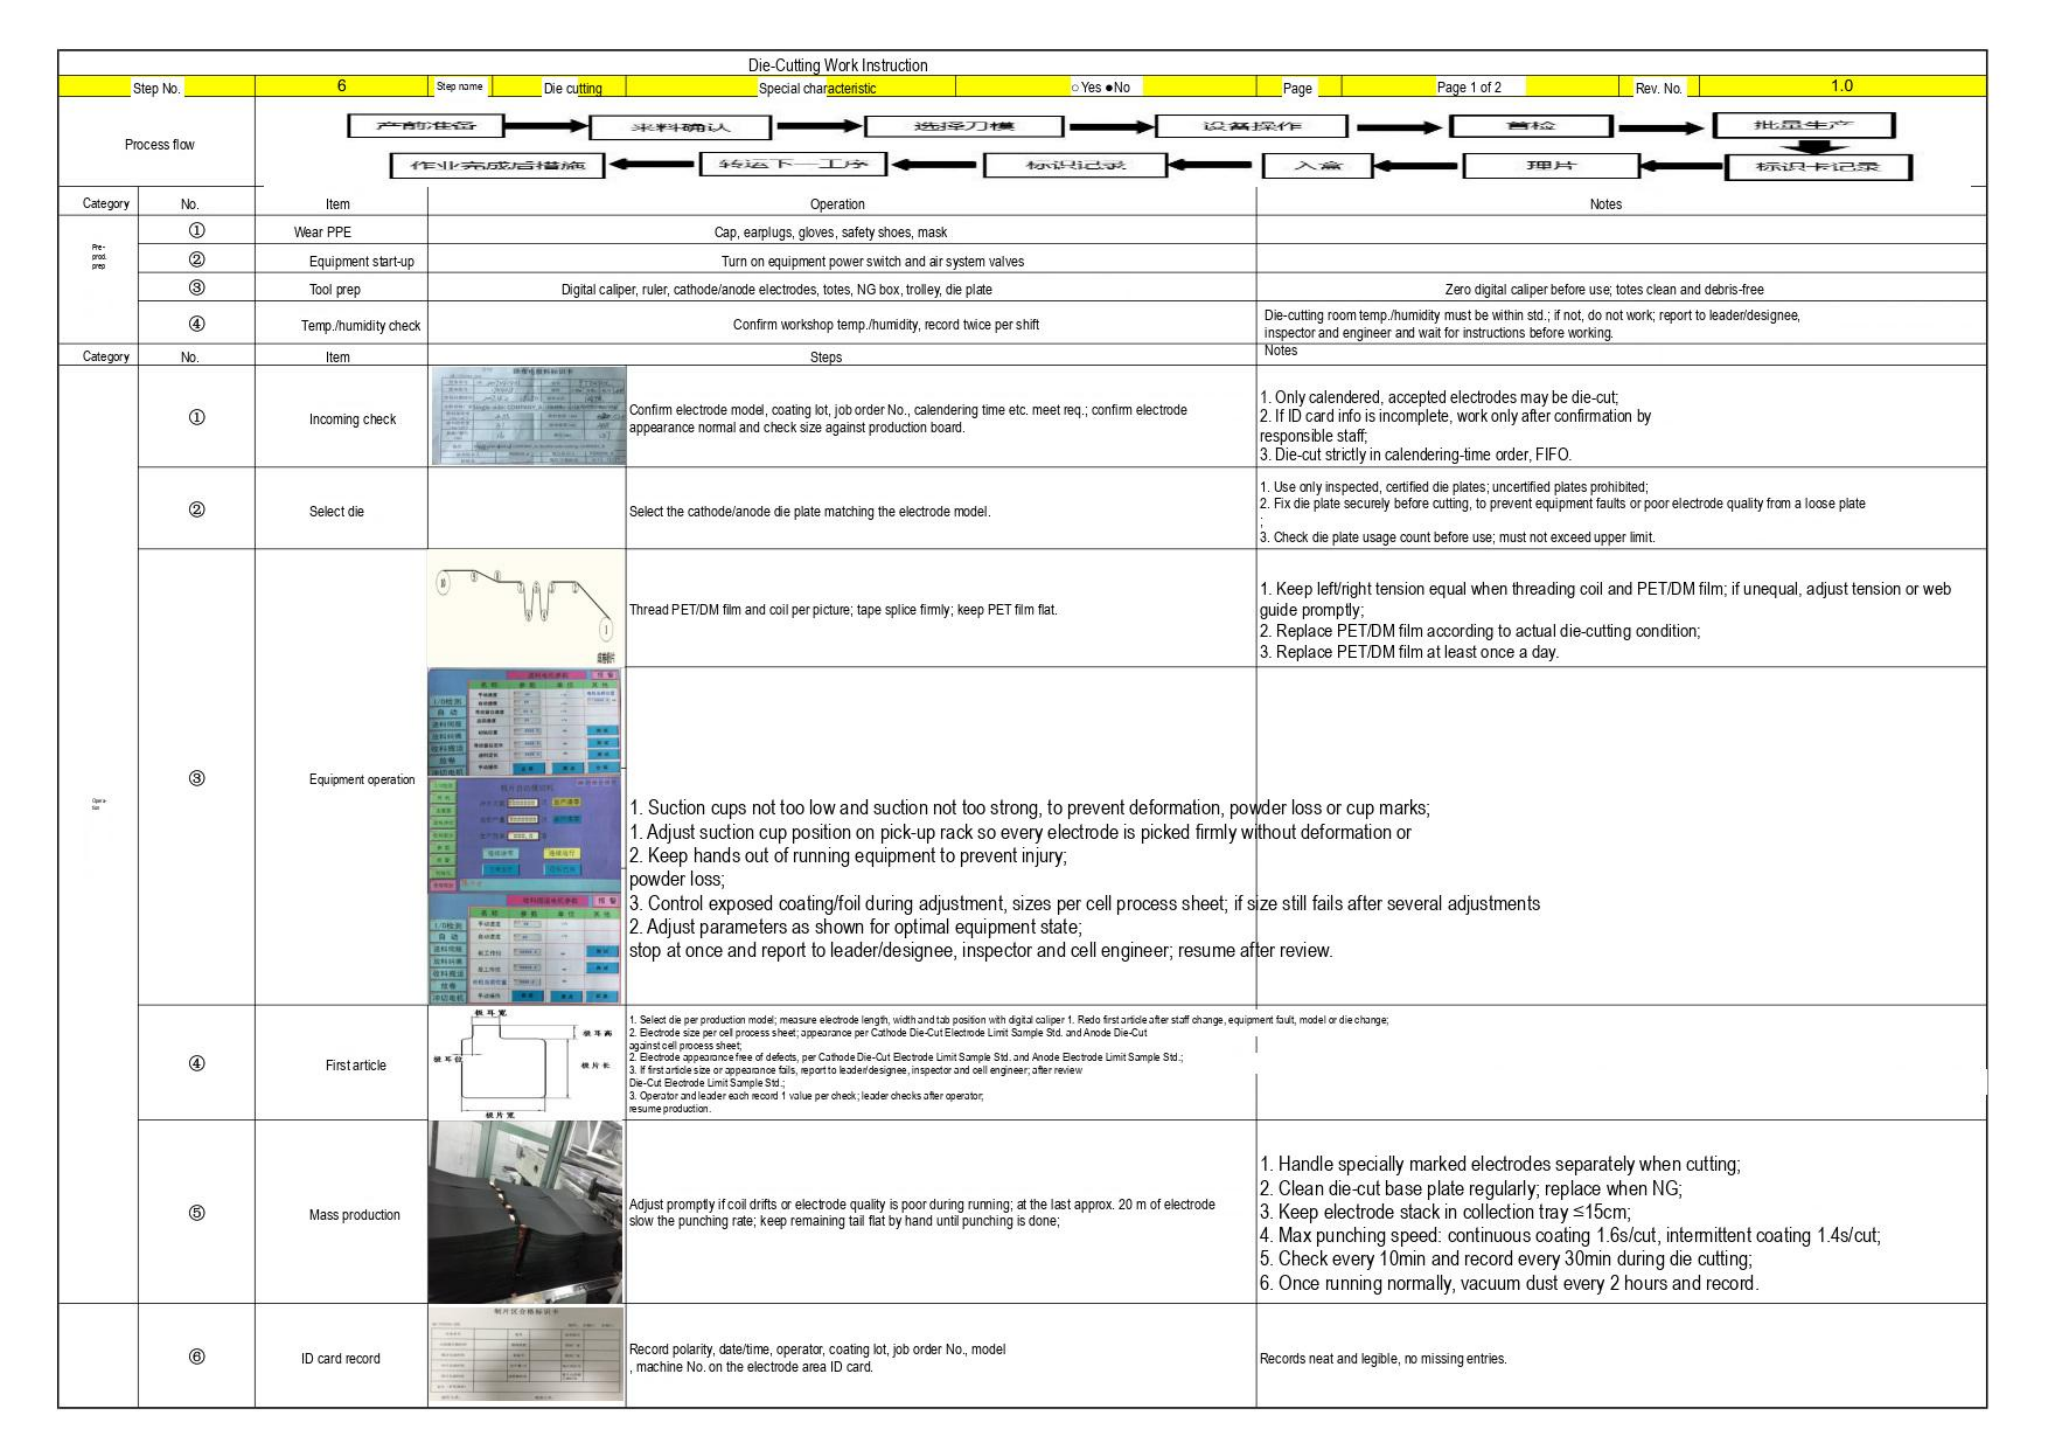Die-Cutting Work Instruction

| Step No. | 6 | Step name | Die cutting | Special characteristic | ○Yes ●No | Page | Page 1 of 2 | Rev. No. | 1.0 |
|---|---|---|---|---|---|---|---|---|---|

Process flow

产前准备 → 来料确认 → 选择刀模 → 设备操作 → 首检 → 批量生产 → 标识卡记录 → 理片 → 入篮 → 标识记录 → 转运下一工序 → 作业完成后措施

| Category | No. | Item | Operation | Notes |
|---|---|---|---|---|
| Pre-prod. prep | ① | Wear PPE | Cap, earplugs, gloves, safety shoes, mask | |
| | ② | Equipment start-up | Turn on equipment power switch and air system valves | |
| | ③ | Tool prep | Digital caliper, ruler, cathode/anode electrodes, totes, NG box, trolley, die plate | Zero digital caliper before use; totes clean and debris-free |
| | ④ | Temp./humidity check | Confirm workshop temp./humidity, record twice per shift | Die-cutting room temp./humidity must be within std.; if not, do not work; report to leader/designee, inspector and engineer and wait for instructions before working. |

| Category | No. | Item | Steps | Notes |
|---|---|---|---|---|
| | ① | Incoming check | Confirm electrode model, coating lot, job order No., calendering time etc. meet req.; confirm electrode appearance normal and check size against production board. | 1. Only calendered, accepted electrodes may be die-cut;<br>2. If ID card info is incomplete, work only after confirmation by responsible staff;<br>3. Die-cut strictly in calendering-time order, FIFO. |
| | ② | Select die | Select the cathode/anode die plate matching the electrode model. | 1. Use only inspected, certified die plates; uncertified plates prohibited;<br>2. Fix die plate securely before cutting, to prevent equipment faults or poor electrode quality from a loose plate<br>;<br>3. Check die plate usage count before use; must not exceed upper limit. |
| | ③ | Equipment operation | Thread PET/DM film and coil per picture; tape splice firmly; keep PET film flat. | 1. Keep left/right tension equal when threading coil and PET/DM film; if unequal, adjust tension or web guide promptly;<br>2. Replace PET/DM film according to actual die-cutting condition;<br>3. Replace PET/DM film at least once a day. |
| | | | 1. Suction cups not too low and suction not too strong, to prevent deformation, powder loss or cup marks;<br>1. Adjust suction cup position on pick-up rack so every electrode is picked firmly without deformation or<br>2. Keep hands out of running equipment to prevent injury;<br>powder loss;<br>3. Control exposed coating/foil during adjustment, sizes per cell process sheet; if size still fails after several adjustments<br>2. Adjust parameters as shown for optimal equipment state;<br>stop at once and report to leader/designee, inspector and cell engineer; resume after review. | |
| | ④ | First article | 极耳宽<br>极耳高<br>极耳位<br>极片长<br>极片宽<br>1. Select die per production model; measure electrode length, width and tab position with digital caliper 1. Redo first article after staff change, equipment fault, model or die change;<br>2. Electrode size per cell process sheet; appearance per Cathode Die-Cut Electrode Limit Sample Std. and Anode Die-Cut<br>against cell process sheet;<br>2. Electrode appearance free of defects, per Cathode Die-Cut Electrode Limit Sample Std. and Anode Electrode Limit Sample Std.;<br>3. If first article size or appearance fails, report to leader/designee, inspector and cell engineer; after review<br>Die-Cut Electrode Limit Sample Std.;<br>3. Operator and leader each record 1 value per check; leader checks after operator;<br>resume production. | |
| | ⑤ | Mass production | Adjust promptly if coil drifts or electrode quality is poor during running; at the last approx. 20 m of electrode slow the punching rate; keep remaining tail flat by hand until punching is done; | 1. Handle specially marked electrodes separately when cutting;<br>2. Clean die-cut base plate regularly; replace when NG;<br>3. Keep electrode stack in collection tray ≤15cm;<br>4. Max punching speed: continuous coating 1.6s/cut, intermittent coating 1.4s/cut;<br>5. Check every 10min and record every 30min during die cutting;<br>6. Once running normally, vacuum dust every 2 hours and record. |
| | ⑥ | ID card record | Record polarity, date/time, operator, coating lot, job order No., model<br>, machine No. on the electrode area ID card. | Records neat and legible, no missing entries. |
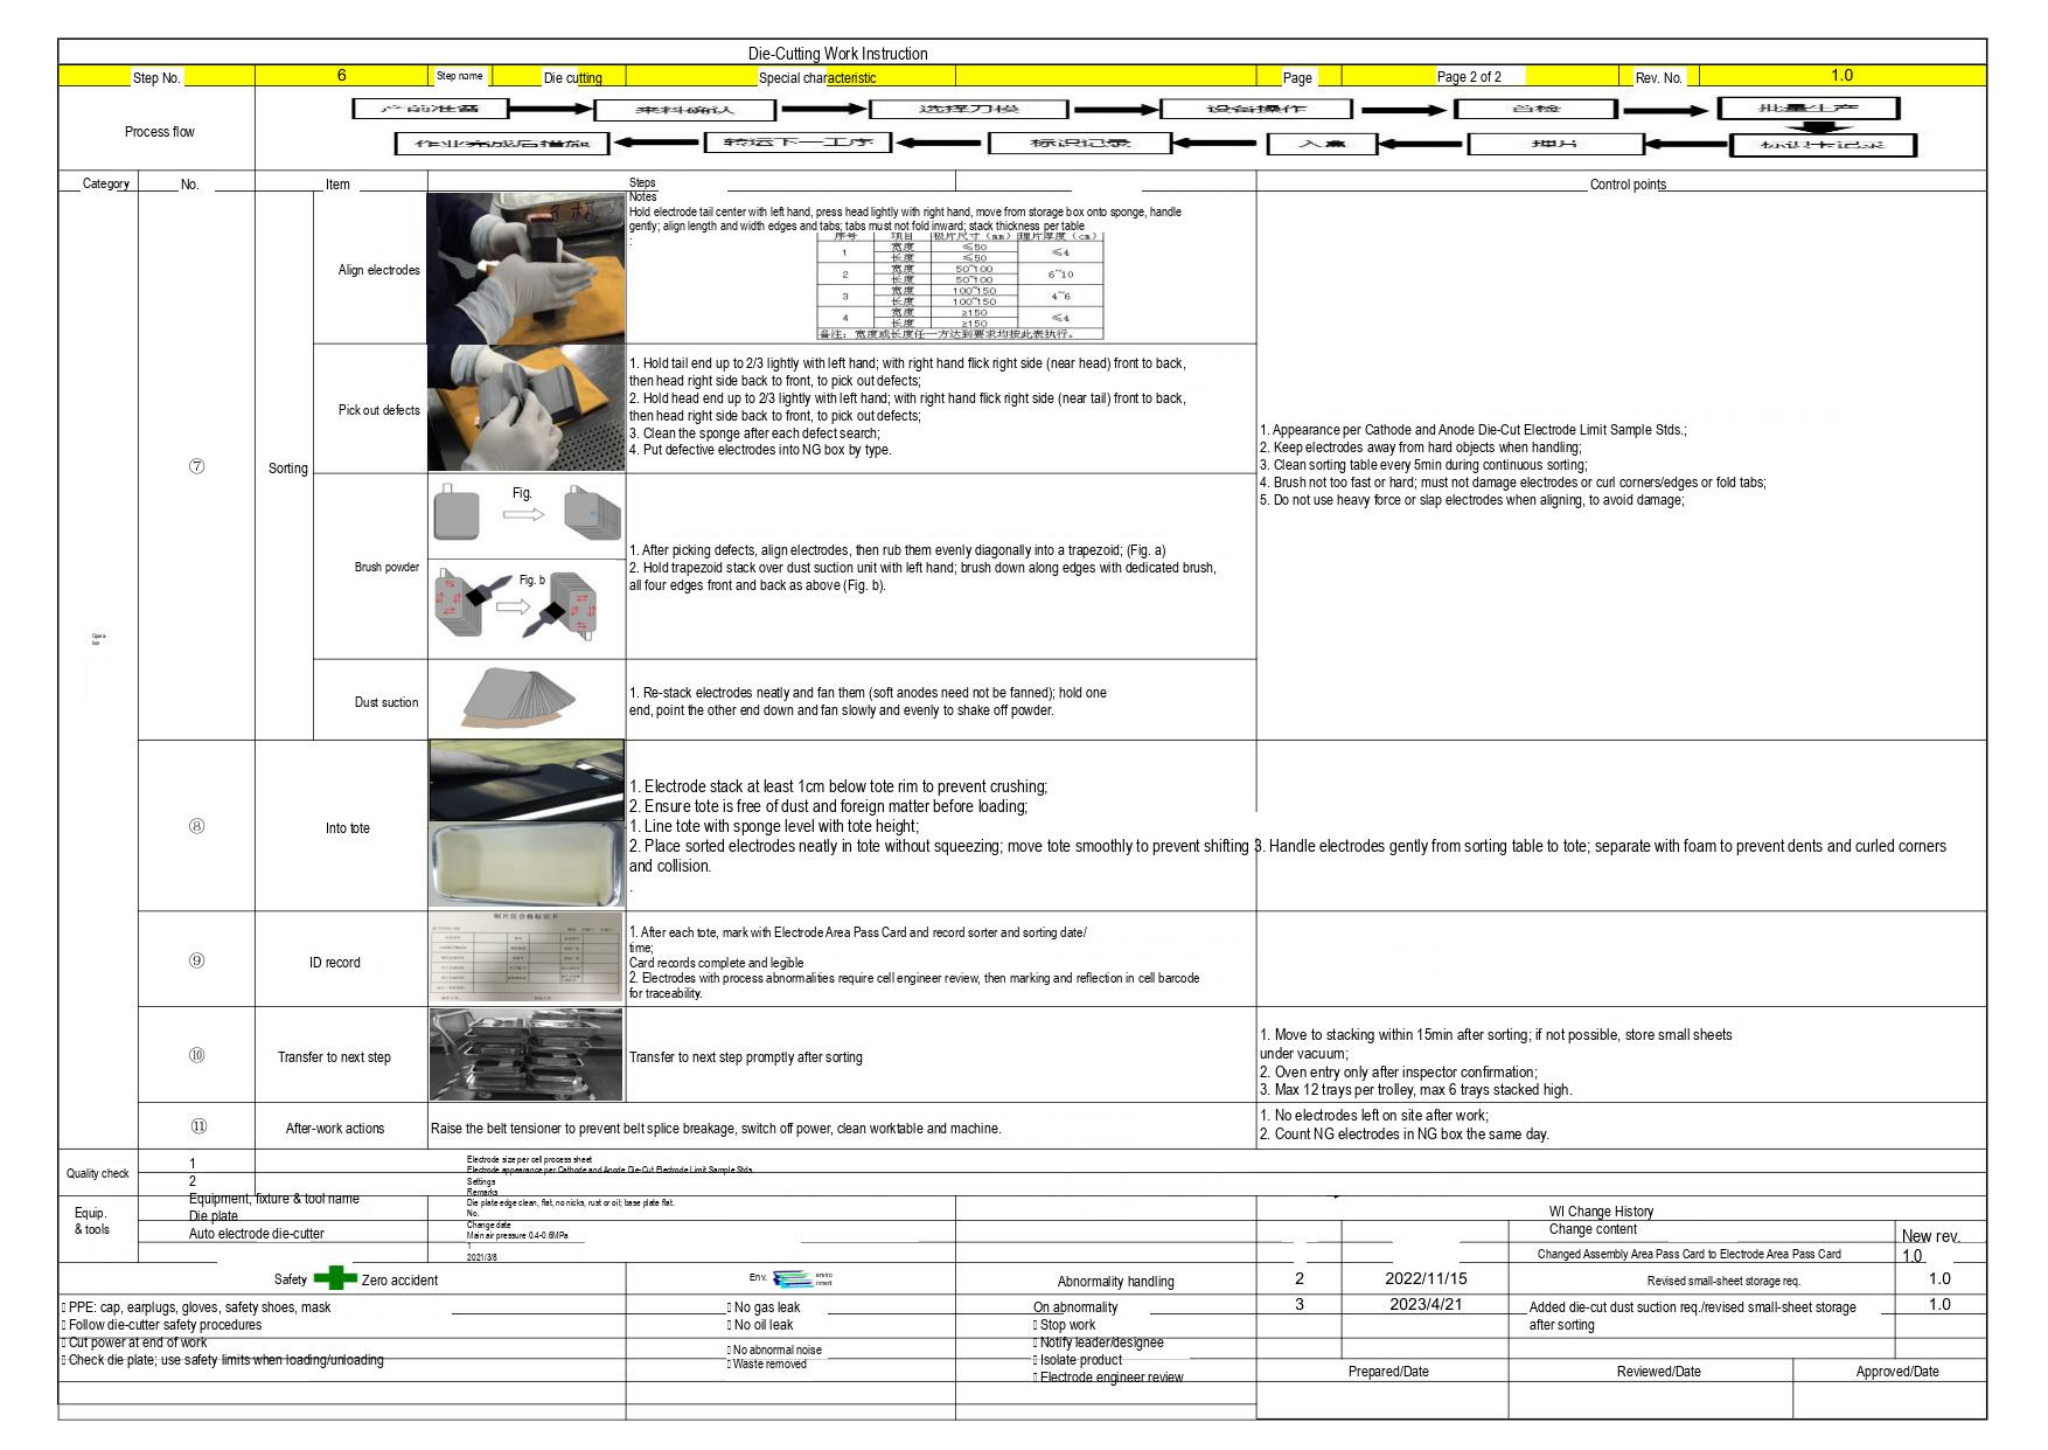# Die-Cutting Work Instruction

| Step No. | 6 | Step name | Die cutting | Special characteristic | | Page | Page 2 of 2 | Rev. No. | 1.0 |
|---|---|---|---|---|---|---|---|---|---|

**Process flow**

来料确认 → 选择刀模 → 设备操作 → 自检 → 批量生产

作业完成后措施 ← 转运下一工序 ← 标识记录 ← 入库 ← 抽片

| Category | No. | Item | | Steps / Notes | Control points |
|---|---|---|---|---|---|
| | ⑦ | Sorting | Align electrodes | Hold electrode tail center with left hand, press head lightly with right hand, move from storage box onto sponge, handle gently; align length and width edges and tabs; tabs must not fold inward; stack thickness per table: | 1. Appearance per Cathode and Anode Die-Cut Electrode Limit Sample Stds.;<br>2. Keep electrodes away from hard objects when handling;<br>3. Clean sorting table every 5min during continuous sorting;<br>4. Brush not too fast or hard; must not damage electrodes or curl corners/edges or fold tabs;<br>5. Do not use heavy force or slap electrodes when aligning, to avoid damage; |
| | | | Pick out defects | 1. Hold tail end up to 2/3 lightly with left hand; with right hand flick right side (near head) front to back, then head right side back to front, to pick out defects;<br>2. Hold head end up to 2/3 lightly with left hand; with right hand flick right side (near tail) front to back, then head right side back to front, to pick out defects;<br>3. Clean the sponge after each defect search;<br>4. Put defective electrodes into NG box by type. | |
| | | | Brush powder | Fig.<br>Fig. b<br>1. After picking defects, align electrodes, then rub them evenly diagonally into a trapezoid; (Fig. a)<br>2. Hold trapezoid stack over dust suction unit with left hand; brush down along edges with dedicated brush, all four edges front and back as above (Fig. b). | |
| | | | Dust suction | 1. Re-stack electrodes neatly and fan them (soft anodes need not be fanned); hold one end, point the other end down and fan slowly and evenly to shake off powder. | |
| | ⑧ | Into tote | | 1. Electrode stack at least 1cm below tote rim to prevent crushing;<br>2. Ensure tote is free of dust and foreign matter before loading;<br>1. Line tote with sponge level with tote height;<br>2. Place sorted electrodes neatly in tote without squeezing; move tote smoothly to prevent shifting and collision. | 3. Handle electrodes gently from sorting table to tote; separate with foam to prevent dents and curled corners |
| | ⑨ | ID record | | 1. After each tote, mark with Electrode Area Pass Card and record sorter and sorting date/ time;<br>Card records complete and legible<br>2. Electrodes with process abnormalities require cell engineer review, then marking and reflection in cell barcode for traceability. | |
| | ⑩ | Transfer to next step | | Transfer to next step promptly after sorting | 1. Move to stacking within 15min after sorting; if not possible, store small sheets under vacuum;<br>2. Oven entry only after inspector confirmation;<br>3. Max 12 trays per trolley, max 6 trays stacked high. |
| | ⑪ | After-work actions | | Raise the belt tensioner to prevent belt splice breakage, switch off power, clean worktable and machine. | 1. No electrodes left on site after work;<br>2. Count NG electrodes in NG box the same day. |

Stack thickness table (Align electrodes):

| 序号 | 项目 | 极片尺寸（mm） | 堆片厚度（cm） |
|---|---|---|---|
| 1 | 宽度 | ≤50 | ≤4 |
| | 长度 | ≤50 | |
| 2 | 宽度 | 50~100 | 6~10 |
| | 长度 | 50~100 | |
| 3 | 宽度 | 100~150 | 4~6 |
| | 长度 | 100~150 | |
| 4 | 宽度 | ≥150 | ≤4 |
| | 长度 | ≥150 | |

备注：宽度或长度任一方达到要求均按此表执行。

| Quality check | 1 | Electrode size per cell process sheet |
|---|---|---|
| | | Electrode appearance per Cathode and Anode Die-Cut Electrode Limit Sample Stds. |
| | 2 | Settings |
| | | Remarks |

| Equip. & tools | Equipment, fixture & tool name | |
|---|---|---|
| | Die plate | Die plate edge clean, flat, no nicks, rust or oil; base plate flat. |
| | Auto electrode die-cutter | Main air pressure 0.4-0.6MPa |

No.
Change date
1
2021/3/8

| Safety Zero accident | Env. | Abnormality handling |
|---|---|---|
| PPE: cap, earplugs, gloves, safety shoes, mask<br>Follow die-cutter safety procedures<br>Cut power at end of work<br>Check die plate; use safety limits when loading/unloading | No gas leak<br>No oil leak<br>No abnormal noise<br>Waste removed | On abnormality<br>Stop work<br>Notify leader/designee<br>Isolate product<br>Electrode engineer review |

WI Change History

| No. | Change date | Change content | New rev. |
|---|---|---|---|
| 1 | 2021/3/8 | Changed Assembly Area Pass Card to Electrode Area Pass Card | 1.0 |
| 2 | 2022/11/15 | Revised small-sheet storage req. | 1.0 |
| 3 | 2023/4/21 | Added die-cut dust suction req./revised small-sheet storage after sorting | 1.0 |

| Prepared/Date | Reviewed/Date | Approved/Date |
|---|---|---|
| | | |